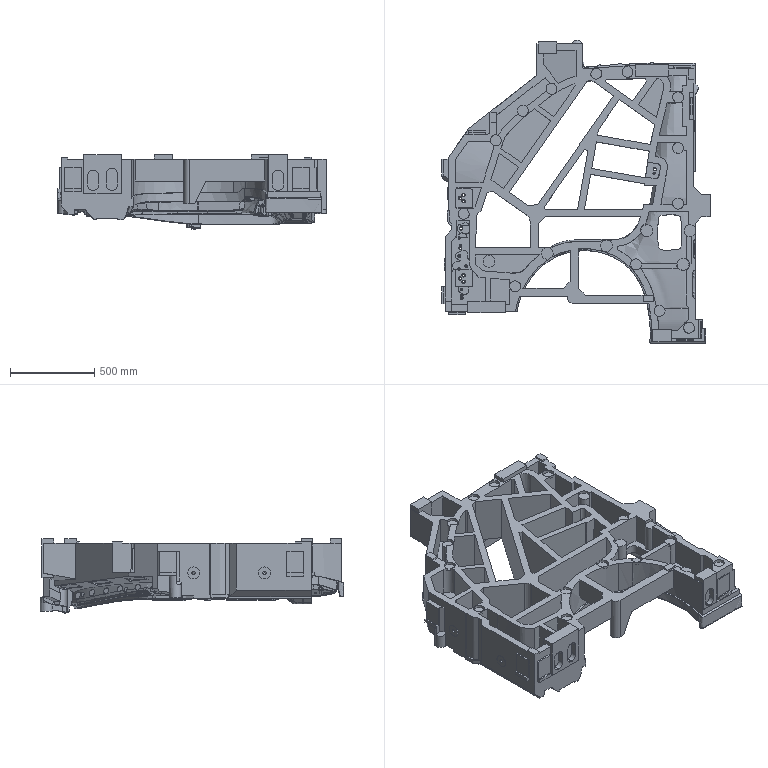Part | NX | features solid 2 | 1 solid | 2696 faces | box 1590 x 1797 x 440.073 mm | volume 255504573 mm3 | spline 1587 | plane 653 | cylinder 429 | cone 10 | torus 9 | sphere 8 | commonest cylinder face diameters 10 x60 20 x45 40 x33 6 x25 14 x25 65 x25